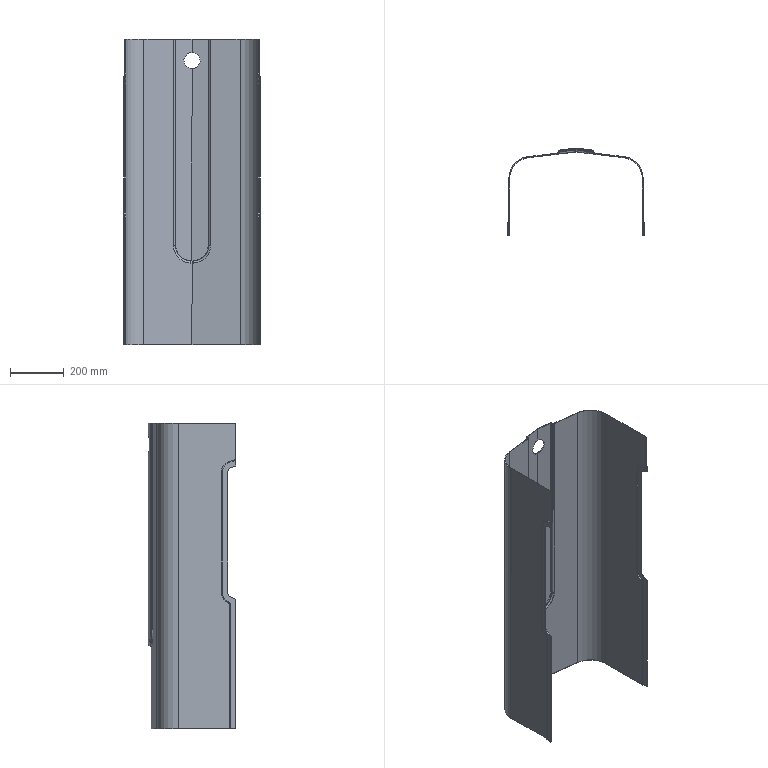Part | SolidWorks | 1 solid | 112 faces | box 510 x 325.072 x 1140 mm | volume 2882610 mm3 | cylinder 50 | plane 48 | spline 8 | torus 6 | commonest cylinder face diameters 7 x8 10 x8 5 x4 15 x4 40 x4 75 x4